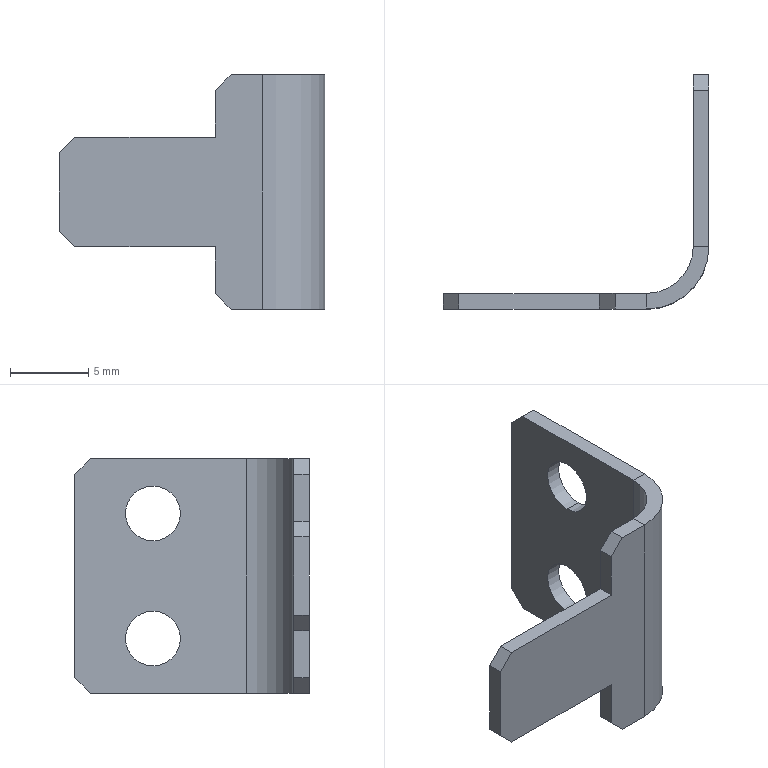Part | STEP file | PN_0031 Sensor BKT_Default | 1 solid | 28 faces | box 17 x 15 x 15 mm | volume 340.225 mm3 | plane 22 | cylinder 6 | commonest cylinder face diameters 3.5 x4 6 x1 8 x1